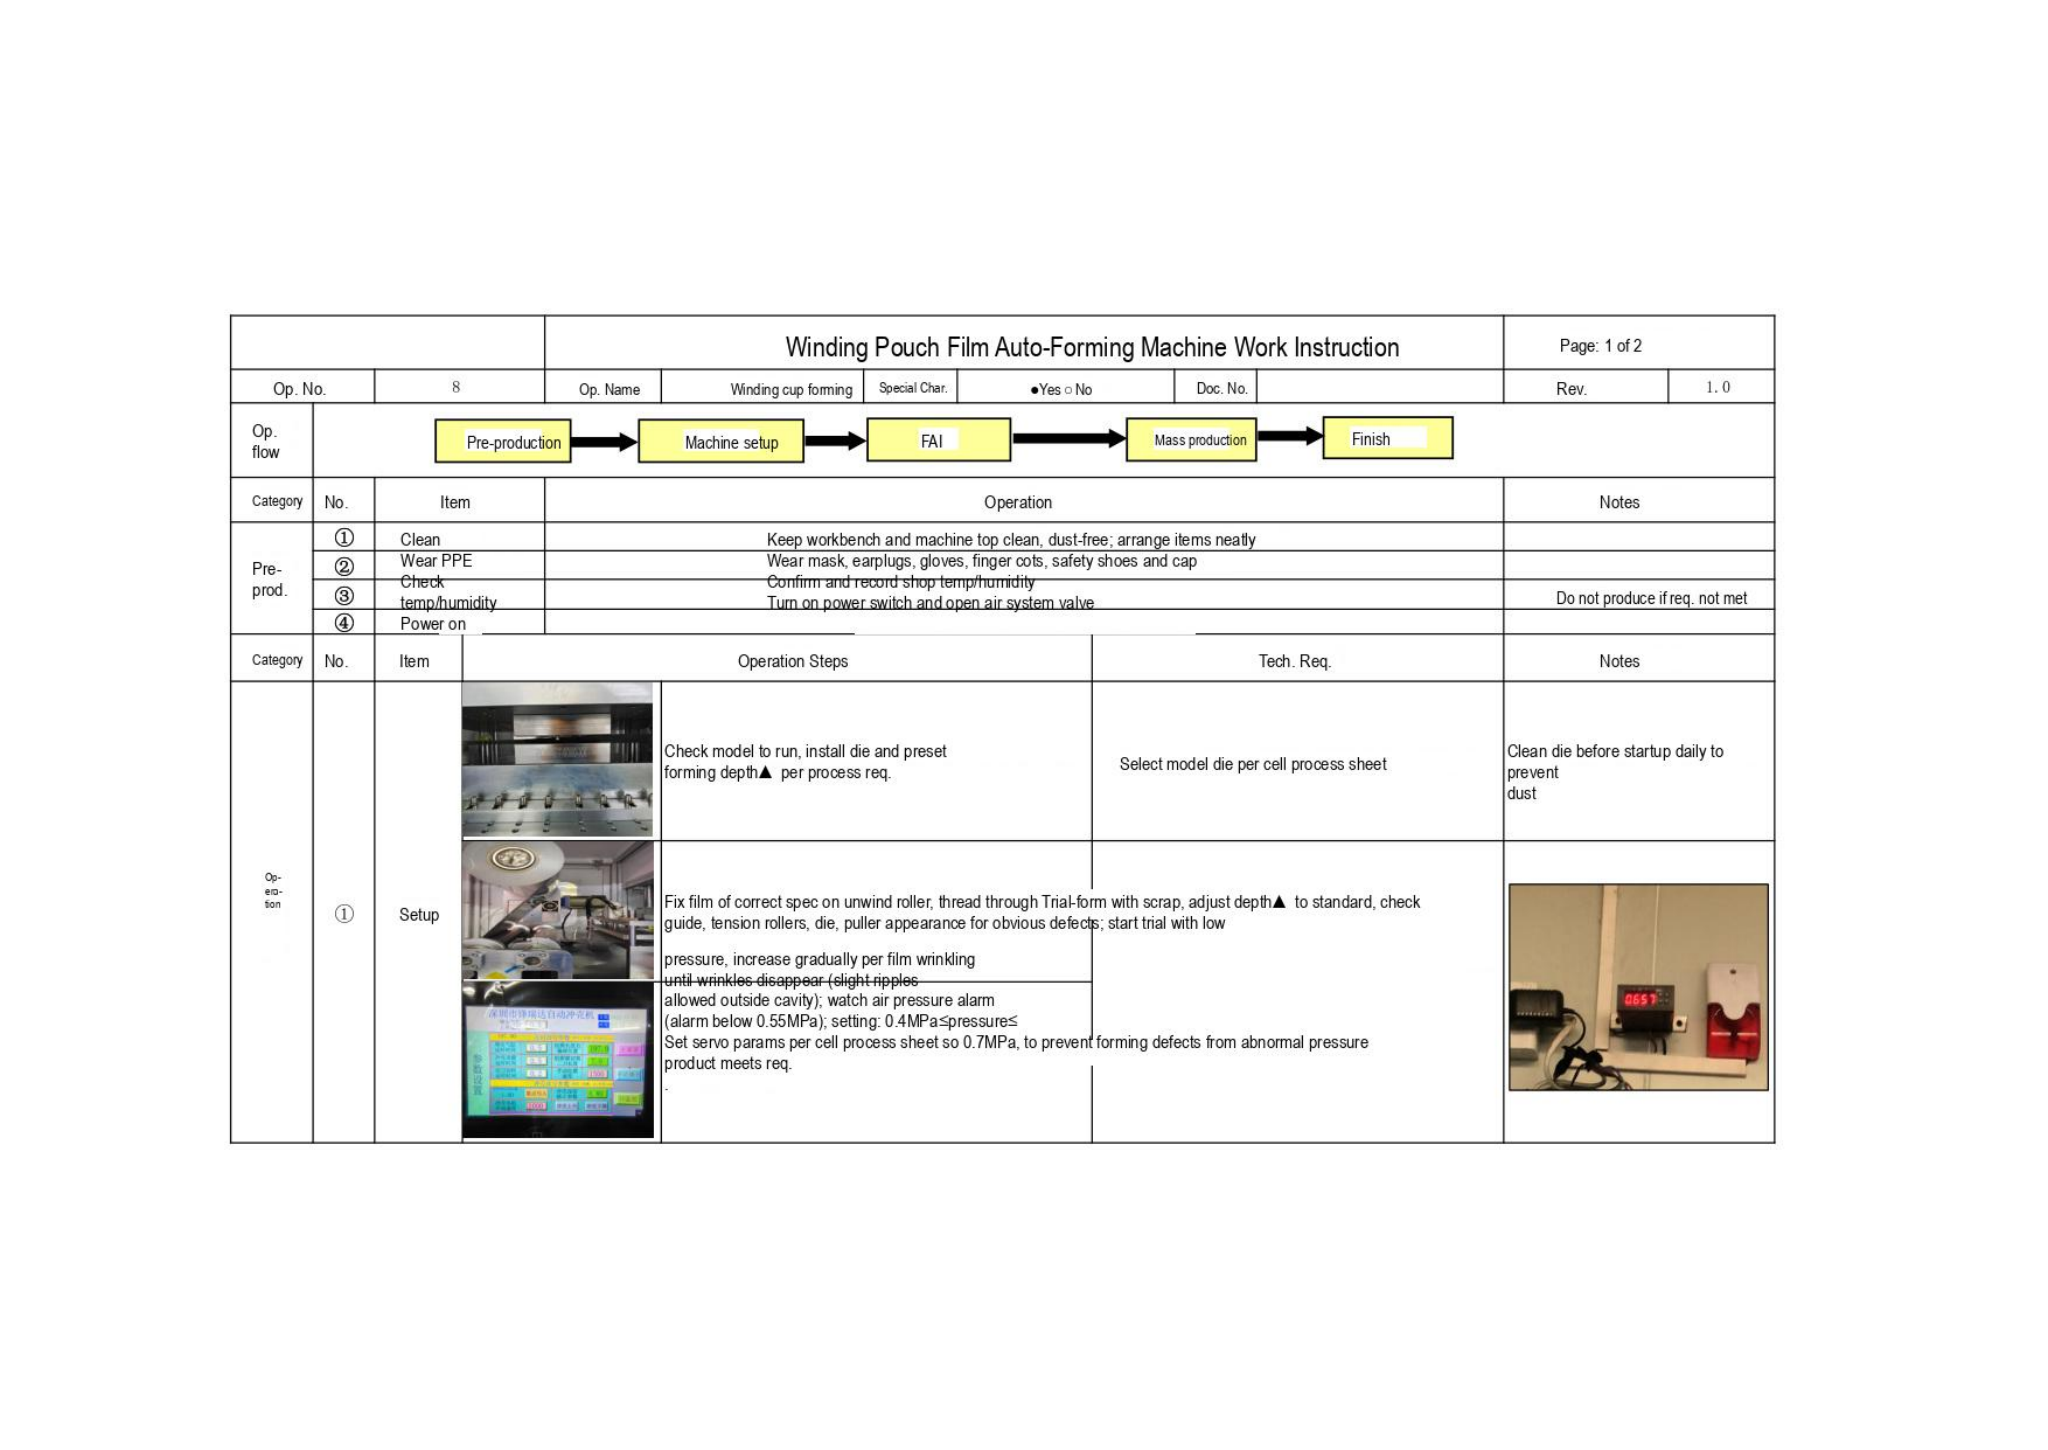# Winding Pouch Film Auto-Forming Machine Work Instruction

| | Winding Pouch Film Auto-Forming Machine Work Instruction | | | | | | | Page: 1 of 2 | |
|---|---|---|---|---|---|---|---|---|---|
| Op. No. | 8 | Op. Name | Winding cup forming | Special Char. | ●Yes ○ No | Doc. No. | | Rev. | 1.0 |

**Op. flow:** Pre-production → Machine setup → FAI → Mass production → Finish

| Category | No. | Item | Operation | Notes |
|---|---|---|---|---|
| Pre-prod. | ① | Clean | Keep workbench and machine top clean, dust-free; arrange items neatly | |
| | ② | Wear PPE | Wear mask, earplugs, gloves, finger cots, safety shoes and cap | |
| | ③ | Check temp/humidity | Confirm and record shop temp/humidity<br>Turn on power switch and open air system valve | Do not produce if req. not met |
| | ④ | Power on | | |

| Category | No. | Item | Operation Steps | Tech. Req. | Notes |
|---|---|---|---|---|---|
| Op-era-tion | ① | Setup | Check model to run, install die and preset forming depth▲ per process req. | Select model die per cell process sheet | Clean die before startup daily to prevent dust |
| | | | Fix film of correct spec on unwind roller, thread through Trial-form with scrap, adjust depth▲ to standard, check guide, tension rollers, die, puller appearance for obvious defects; start trial with low<br><br>pressure, increase gradually per film wrinkling<br>until wrinkles disappear (slight ripples<br>allowed outside cavity); watch air pressure alarm<br>(alarm below 0.55MPa); setting: 0.4MPa≤pressure≤<br>Set servo params per cell process sheet so 0.7MPa, to prevent forming defects from abnormal pressure<br>product meets req. | | 0657 |
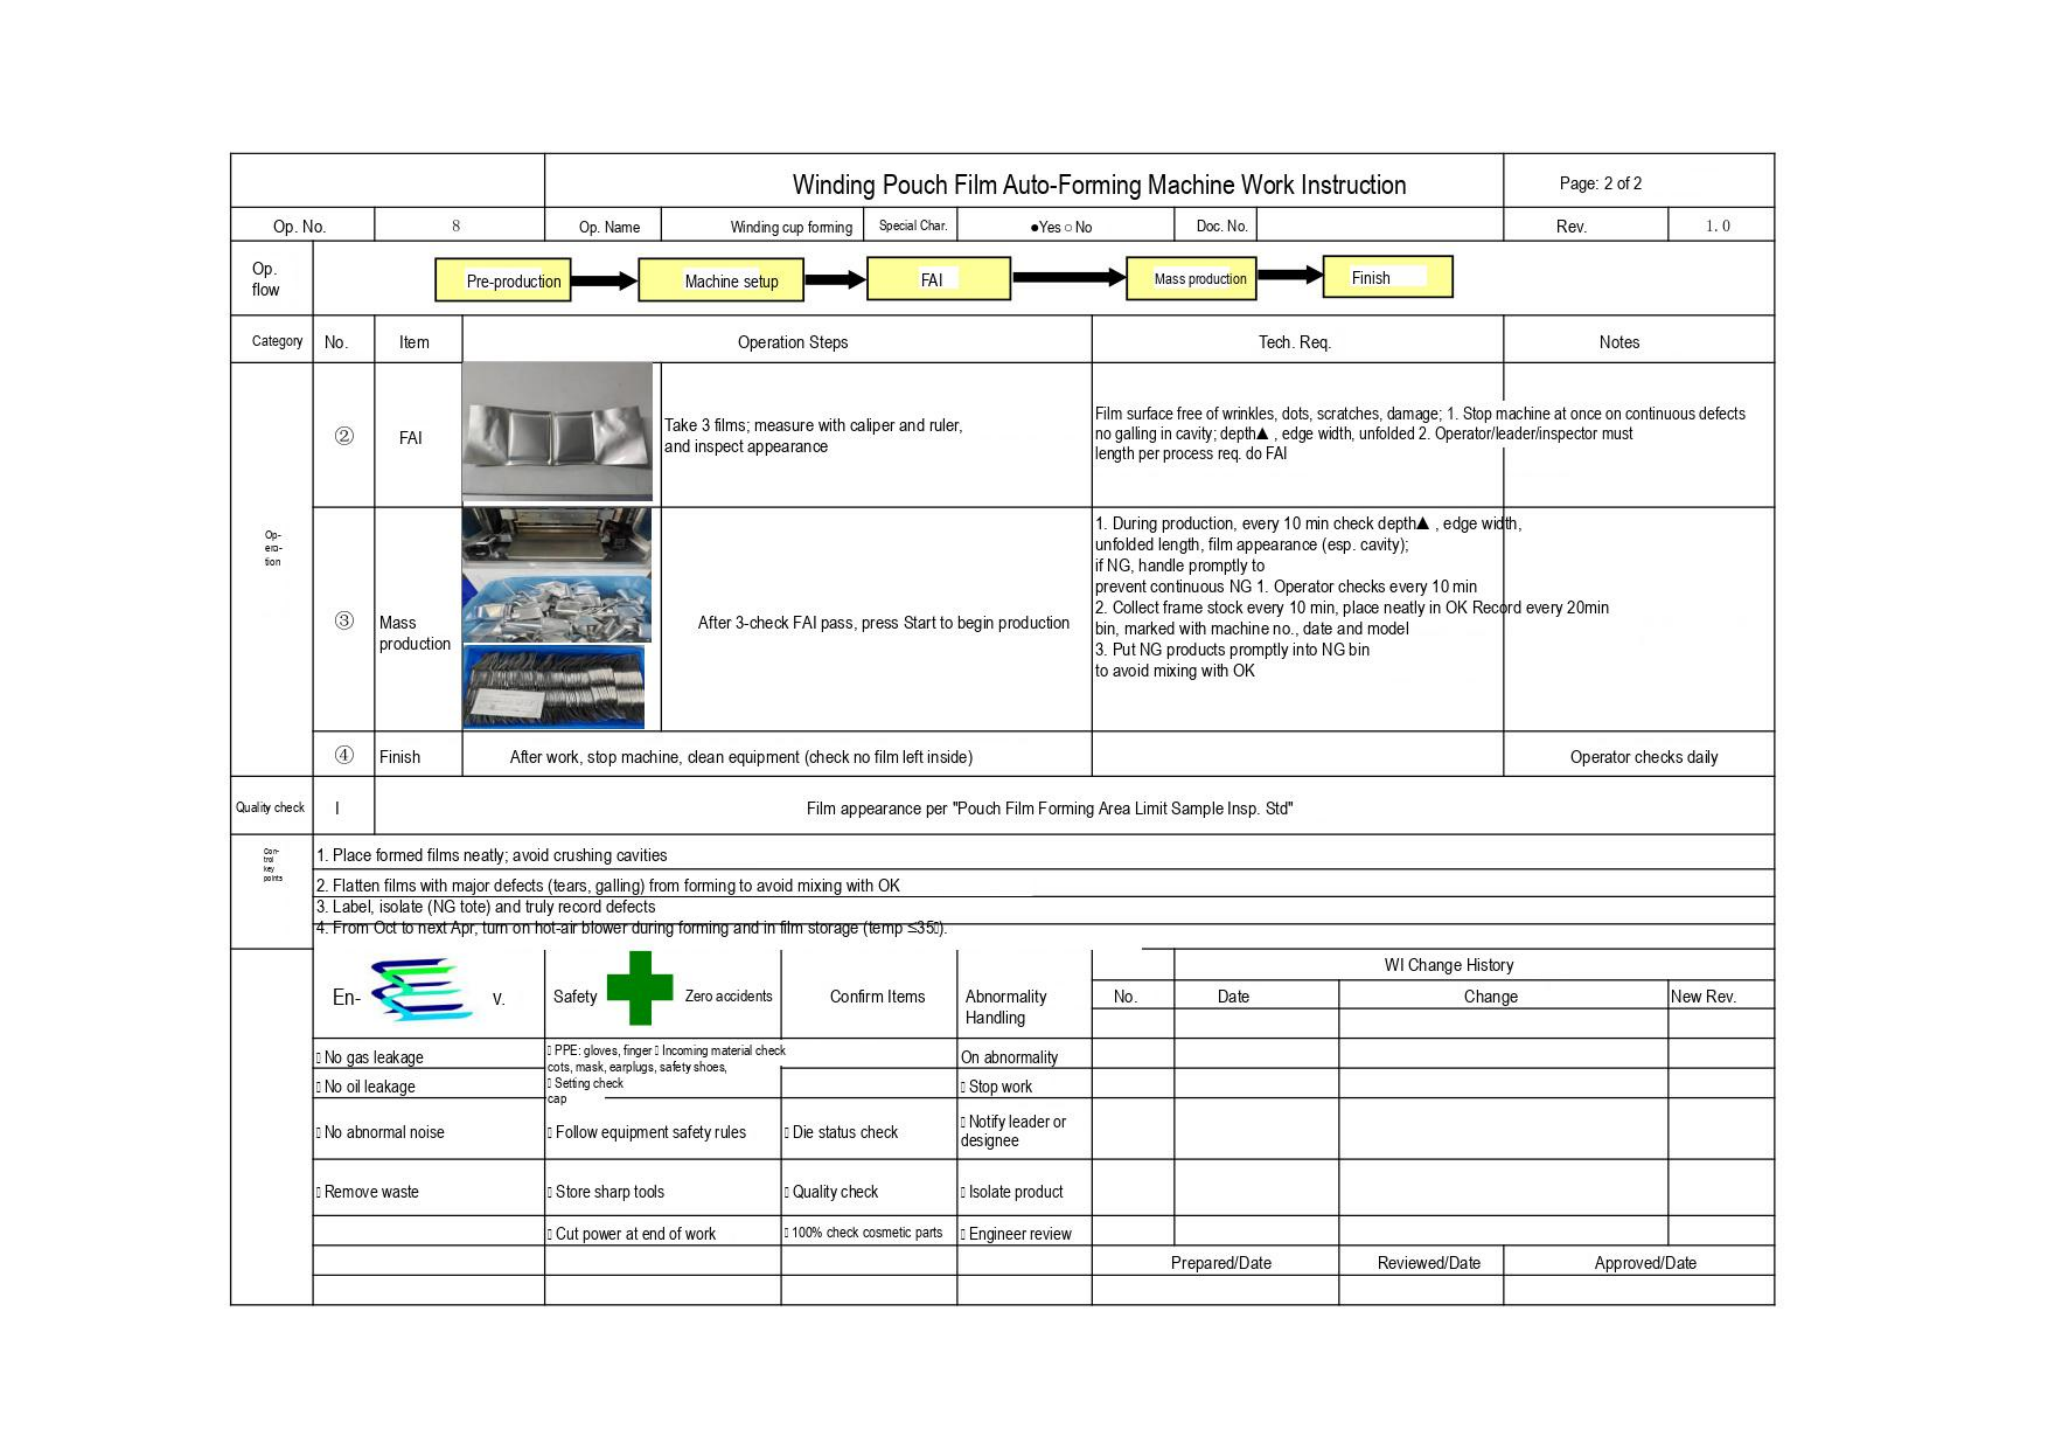# Winding Pouch Film Auto-Forming Machine Work Instruction

Page: 2 of 2

| Op. No. | 8 | Op. Name | Winding cup forming | Special Char. | ●Yes ○ No | Doc. No. | | Rev. | 1.0 |
|---|---|---|---|---|---|---|---|---|---|

Op. flow: Pre-production → Machine setup → FAI → Mass production → Finish

| Category | No. | Item | Operation Steps | Tech. Req. | Notes |
|---|---|---|---|---|---|
| Op-era-tion | ② | FAI | Take 3 films; measure with caliper and ruler, and inspect appearance | Film surface free of wrinkles, dots, scratches, damage; no galling in cavity; depth▲, edge width, unfolded length per process req. | 1. Stop machine at once on continuous defects 2. Operator/leader/inspector must do FAI |
| | ③ | Mass production | After 3-check FAI pass, press Start to begin production | 1. During production, every 10 min check depth▲, edge width, unfolded length, film appearance (esp. cavity); if NG, handle promptly to prevent continuous NG 2. Collect frame stock every 10 min, place neatly in OK bin, marked with machine no., date and model 3. Put NG products promptly into NG bin to avoid mixing with OK | 1. Operator checks every 10 min Record every 20min |
| | ④ | Finish | After work, stop machine, clean equipment (check no film left inside) | | Operator checks daily |
| Quality check | I | Film appearance per "Pouch Film Forming Area Limit Sample Insp. Std" | | | |

| Con-trol key points |
|---|
| 1. Place formed films neatly; avoid crushing cavities |
| 2. Flatten films with major defects (tears, galling) from forming to avoid mixing with OK |
| 3. Label, isolate (NG tote) and truly record defects |
| 4. From Oct to next Apr, turn on hot-air blower during forming and in film storage (temp ≤35▯). |

| En- v. | Safety Zero accidents | Confirm Items | Abnormality Handling |
|---|---|---|---|
| ▯ No gas leakage | ▯ PPE: gloves, finger cots, mask, earplugs, safety shoes, cap | ▯ Incoming material check | On abnormality |
| ▯ No oil leakage | | ▯ Setting check | ▯ Stop work |
| ▯ No abnormal noise | ▯ Follow equipment safety rules | ▯ Die status check | ▯ Notify leader or designee |
| ▯ Remove waste | ▯ Store sharp tools | ▯ Quality check | ▯ Isolate product |
| | ▯ Cut power at end of work | ▯ 100% check cosmetic parts | ▯ Engineer review |

WI Change History

| No. | Date | Change | New Rev. |
|---|---|---|---|
| | | | |

| Prepared/Date | Reviewed/Date | Approved/Date |
|---|---|---|
| | | |